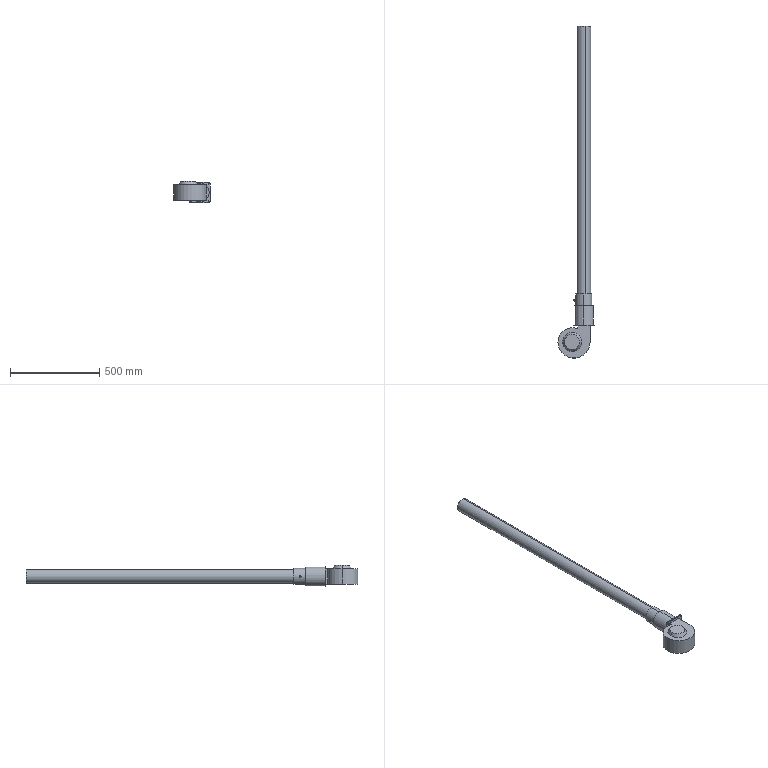Part | SolidWorks | features CompositeCurve 1 | 2 solids | 75 faces | box 202.5 x 1859 x 119.5 mm | volume 4220516 mm3 | cylinder 50 | plane 23 | cone 2 | commonest cylinder face diameters 12 x26 5 x8 20 x4 8 x2 74 x2 76 x2